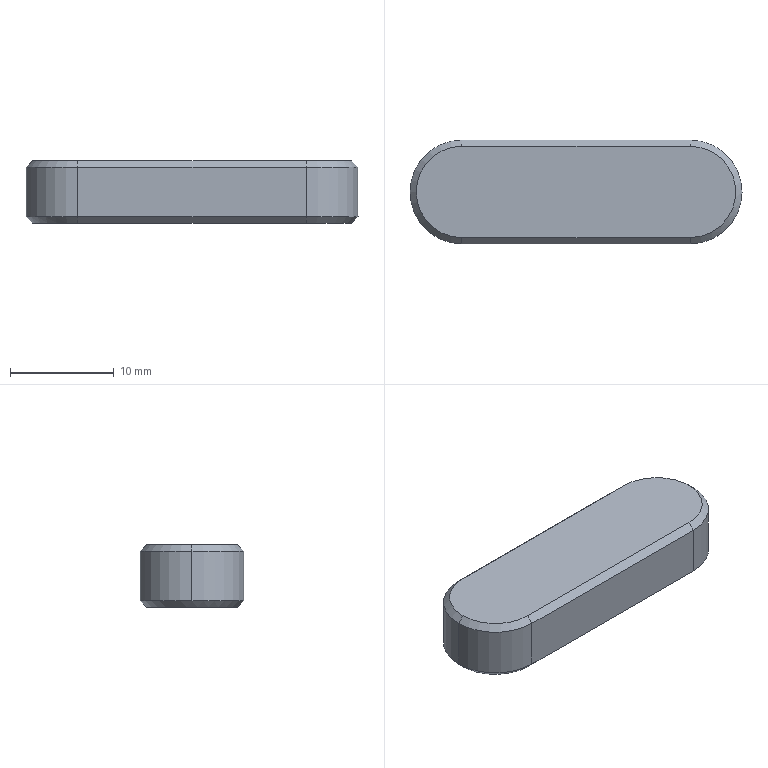Part | SolidWorks | features BaseBody 1 | 1 solid | 17 faces | box 32 x 10 x 6 mm | volume 1765 mm3 | plane 8 | cone 6 | cylinder 3 | commonest cylinder face diameters 10 x3
STEP:
#1=CARTESIAN_POINT('',(0.6,0.,2.5));
#2=VERTEX_POINT('',#1);
#3=CARTESIAN_POINT('',(5.,-4.4,2.5));
#4=VERTEX_POINT('',#3);
#5=CARTESIAN_POINT('',(5.,0.,2.5));
#6=DIRECTION('',(0.,0.,1.));
#7=DIRECTION('',(-1.,0.,0.));
#8=AXIS2_PLACEMENT_3D('',#5,#6,#7);
#9=CIRCLE('',#8,4.4);
#10=EDGE_CURVE('',#2,#4,#9,.T.);
#11=ORIENTED_EDGE('',*,*,#10,.F.);
#12=CARTESIAN_POINT('',(0.,0.,1.9));
#13=VERTEX_POINT('',#12);
#14=CARTESIAN_POINT('',(0.,0.,1.9));
#15=DIRECTION('',(-0.7071,0.,-0.7071));
#16=VECTOR('',#15,1000.);
#17=LINE('',#14,#16);
#18=EDGE_CURVE('',#2,#13,#17,.T.);
#19=ORIENTED_EDGE('',*,*,#18,.T.);
#20=CARTESIAN_POINT('',(5.,-5.,1.9));
#21=VERTEX_POINT('',#20);
#22=CARTESIAN_POINT('',(5.,0.,1.9));
#23=DIRECTION('',(0.,0.,1.));
#24=DIRECTION('',(0.,-1.,0.));
#25=AXIS2_PLACEMENT_3D('',#22,#23,#24);
#26=CIRCLE('',#25,5.);
#27=EDGE_CURVE('',#13,#21,#26,.T.);
#28=ORIENTED_EDGE('',*,*,#27,.T.);
#29=CARTESIAN_POINT('',(5.,-4.7,2.2));
#30=DIRECTION('',(0.,-0.7071,-0.7071));
#31=VECTOR('',#30,1000.);
#32=LINE('',#29,#31);
#33=EDGE_CURVE('',#4,#21,#32,.T.);
#34=ORIENTED_EDGE('',*,*,#33,.F.);
#35=EDGE_LOOP('',(#11,#19,#28,#34));
#36=FACE_OUTER_BOUND('',#35,.T.);
#37=CARTESIAN_POINT('',(5.,0.,1.9));
#38=DIRECTION('',(0.,0.,-1.));
#39=DIRECTION('',(-1.,0.,0.));
#40=AXIS2_PLACEMENT_3D('',#37,#38,#39);
#41=CONICAL_SURFACE('',#40,5.,0.7854);
#42=ADVANCED_FACE('',(#36),#41,.T.);
#43=ORIENTED_EDGE('',*,*,#27,.F.);
#44=CARTESIAN_POINT('',(0.,0.,-2.9));
#45=VERTEX_POINT('',#44);
#46=CARTESIAN_POINT('',(0.,0.,0.));
#47=DIRECTION('',(0.,0.,-1.));
#48=VECTOR('',#47,1000.);
#49=LINE('',#46,#48);
#50=EDGE_CURVE('',#13,#45,#49,.T.);
#51=ORIENTED_EDGE('',*,*,#50,.T.);
#52=CARTESIAN_POINT('',(5.,-5.,-2.9));
#53=VERTEX_POINT('',#52);
#54=CARTESIAN_POINT('',(5.,0.,-2.9));
#55=DIRECTION('',(0.,0.,1.));
#56=DIRECTION('',(-1.,0.,0.));
#57=AXIS2_PLACEMENT_3D('',#54,#55,#56);
#58=CIRCLE('',#57,5.);
#59=EDGE_CURVE('',#45,#53,#58,.T.);
#60=ORIENTED_EDGE('',*,*,#59,.T.);
#61=CARTESIAN_POINT('',(5.,-5.,0.));
#62=DIRECTION('',(0.,0.,-1.));
#63=VECTOR('',#62,1000.);
#64=LINE('',#61,#63);
#65=EDGE_CURVE('',#21,#53,#64,.T.);
#66=ORIENTED_EDGE('',*,*,#65,.F.);
#67=EDGE_LOOP('',(#43,#51,#60,#66));
#68=FACE_OUTER_BOUND('',#67,.T.);
#69=CARTESIAN_POINT('',(5.,0.,0.));
#70=DIRECTION('',(0.,0.,-1.));
#71=DIRECTION('',(-1.,0.,0.));
#72=AXIS2_PLACEMENT_3D('',#69,#70,#71);
#73=CYLINDRICAL_SURFACE('',#72,5.);
#74=ADVANCED_FACE('',(#68),#73,.T.);
#75=CARTESIAN_POINT('',(27.,-4.4,-3.5));
#76=VERTEX_POINT('',#75);
#77=CARTESIAN_POINT('',(31.4,0.,-3.5));
#78=VERTEX_POINT('',#77);
#79=CARTESIAN_POINT('',(27.,0.,-3.5));
#80=DIRECTION('',(0.,0.,1.));
#81=DIRECTION('',(1.,0.,0.));
#82=AXIS2_PLACEMENT_3D('',#79,#80,#81);
#83=CIRCLE('',#82,4.4);
#84=EDGE_CURVE('',#76,#78,#83,.T.);
#85=ORIENTED_EDGE('',*,*,#84,.T.);
#86=CARTESIAN_POINT('',(32.,0.,-2.9));
#87=VERTEX_POINT('',#86);
#88=CARTESIAN_POINT('',(32.,0.,-2.9));
#89=DIRECTION('',(0.7071,0.,0.7071));
#90=VECTOR('',#89,1000.);
#91=LINE('',#88,#90);
#92=EDGE_CURVE('',#78,#87,#91,.T.);
#93=ORIENTED_EDGE('',*,*,#92,.T.);
#94=CARTESIAN_POINT('',(27.,-5.,-2.9));
#95=VERTEX_POINT('',#94);
#96=CARTESIAN_POINT('',(27.,0.,-2.9));
#97=DIRECTION('',(0.,0.,1.));
#98=DIRECTION('',(-1.,0.,0.));
#99=AXIS2_PLACEMENT_3D('',#96,#97,#98);
#100=CIRCLE('',#99,5.);
#101=EDGE_CURVE('',#95,#87,#100,.T.);
#102=ORIENTED_EDGE('',*,*,#101,.F.);
#103=CARTESIAN_POINT('',(27.,-499000.,498992.1));
#104=DIRECTION('',(0.,0.7071,-0.7071));
#105=VECTOR('',#104,1000.);
#106=LINE('',#103,#105);
#107=EDGE_CURVE('',#95,#76,#106,.T.);
#108=ORIENTED_EDGE('',*,*,#107,.T.);
#109=EDGE_LOOP('',(#85,#93,#102,#108));
#110=FACE_OUTER_BOUND('',#109,.T.);
#111=CARTESIAN_POINT('',(27.,0.,-2.9));
#112=DIRECTION('',(0.,0.,1.));
#113=DIRECTION('',(1.,0.,0.));
#114=AXIS2_PLACEMENT_3D('',#111,#112,#113);
#115=CONICAL_SURFACE('',#114,5.,0.7854);
#116=ADVANCED_FACE('',(#110),#115,.T.);
#117=CARTESIAN_POINT('',(27.,-4.4,2.5));
#118=VERTEX_POINT('',#117);
#119=CARTESIAN_POINT('',(27.,4.4,2.5));
#120=VERTEX_POINT('',#119);
#121=CARTESIAN_POINT('',(27.,0.,2.5));
#122=DIRECTION('',(0.,0.,1.));
#123=DIRECTION('',(-1.,0.,0.));
#124=AXIS2_PLACEMENT_3D('',#121,#122,#123);
#125=CIRCLE('',#124,4.4);
#126=EDGE_CURVE('',#118,#120,#125,.T.);
#127=ORIENTED_EDGE('',*,*,#126,.T.);
#128=CARTESIAN_POINT('',(5.,4.4,2.5));
#129=VERTEX_POINT('',#128);
#130=CARTESIAN_POINT('',(16.,4.4,2.5));
#131=DIRECTION('',(-1.,0.,0.));
#132=VECTOR('',#131,1000.);
#133=LINE('',#130,#132);
#134=EDGE_CURVE('',#120,#129,#133,.T.);
#135=ORIENTED_EDGE('',*,*,#134,.T.);
#136=CARTESIAN_POINT('',(5.,0.,2.5));
#137=DIRECTION('',(0.,0.,1.));
#138=DIRECTION('',(-1.,0.,0.));
#139=AXIS2_PLACEMENT_3D('',#136,#137,#138);
#140=CIRCLE('',#139,4.4);
#141=EDGE_CURVE('',#129,#2,#140,.T.);
#142=ORIENTED_EDGE('',*,*,#141,.T.);
#143=ORIENTED_EDGE('',*,*,#10,.T.);
#144=CARTESIAN_POINT('',(16.,-4.4,2.5));
#145=DIRECTION('',(1.,0.,0.));
#146=VECTOR('',#145,1000.);
#147=LINE('',#144,#146);
#148=EDGE_CURVE('',#4,#118,#147,.T.);
#149=ORIENTED_EDGE('',*,*,#148,.T.);
#150=EDGE_LOOP('',(#127,#135,#142,#143,#149));
#151=FACE_OUTER_BOUND('',#150,.T.);
#152=CARTESIAN_POINT('',(16.,0.,2.5));
#153=DIRECTION('',(0.,0.,1.));
#154=DIRECTION('',(1.,0.,0.));
#155=AXIS2_PLACEMENT_3D('',#152,#153,#154);
#156=PLANE('',#155);
#157=ADVANCED_FACE('',(#151),#156,.T.);
#158=CARTESIAN_POINT('',(5.,5.,1.9));
#159=VERTEX_POINT('',#158);
#160=CARTESIAN_POINT('',(5.,4.7,2.2));
#161=DIRECTION('',(0.,-0.7071,0.7071));
#162=VECTOR('',#161,1000.);
#163=LINE('',#160,#162);
#164=EDGE_CURVE('',#159,#129,#163,.T.);
#165=ORIENTED_EDGE('',*,*,#164,.T.);
#166=ORIENTED_EDGE('',*,*,#134,.F.);
#167=CARTESIAN_POINT('',(27.,5.,1.9));
#168=VERTEX_POINT('',#167);
#169=CARTESIAN_POINT('',(27.,4.7,2.2));
#170=DIRECTION('',(0.,0.7071,-0.7071));
#171=VECTOR('',#170,1000.);
#172=LINE('',#169,#171);
#173=EDGE_CURVE('',#120,#168,#172,.T.);
#174=ORIENTED_EDGE('',*,*,#173,.T.);
#175=CARTESIAN_POINT('',(21.5,5.,1.9));
#176=DIRECTION('',(-1.,0.,0.));
#177=VECTOR('',#176,1000.);
#178=LINE('',#175,#177);
#179=EDGE_CURVE('',#168,#159,#178,.T.);
#180=ORIENTED_EDGE('',*,*,#179,.T.);
#181=EDGE_LOOP('',(#165,#166,#174,#180));
#182=FACE_OUTER_BOUND('',#181,.T.);
#183=CARTESIAN_POINT('',(21.5,4.7,2.2));
#184=DIRECTION('',(0.,0.7071,0.7071));
#185=DIRECTION('',(0.,-0.7071,0.7071));
#186=AXIS2_PLACEMENT_3D('',#183,#184,#185);
#187=PLANE('',#186);
#188=ADVANCED_FACE('',(#182),#187,.T.);
#189=ORIENTED_EDGE('',*,*,#173,.F.);
#190=ORIENTED_EDGE('',*,*,#126,.F.);
#191=CARTESIAN_POINT('',(27.,-5.,1.9));
#192=VERTEX_POINT('',#191);
#193=CARTESIAN_POINT('',(27.,-499000.,-498993.1));
#194=DIRECTION('',(0.,-0.7071,-0.7071));
#195=VECTOR('',#194,1000.);
#196=LINE('',#193,#195);
#197=EDGE_CURVE('',#118,#192,#196,.T.);
#198=ORIENTED_EDGE('',*,*,#197,.T.);
#199=CARTESIAN_POINT('',(27.,0.,1.9));
#200=DIRECTION('',(0.,0.,1.));
#201=DIRECTION('',(0.,1.,0.));
#202=AXIS2_PLACEMENT_3D('',#199,#200,#201);
#203=CIRCLE('',#202,5.);
#204=EDGE_CURVE('',#192,#168,#203,.T.);
#205=ORIENTED_EDGE('',*,*,#204,.T.);
#206=EDGE_LOOP('',(#189,#190,#198,#205));
#207=FACE_OUTER_BOUND('',#206,.T.);
#208=CARTESIAN_POINT('',(27.,0.,1.9));
#209=DIRECTION('',(0.,0.,-1.));
#210=DIRECTION('',(-1.,0.,0.));
#211=AXIS2_PLACEMENT_3D('',#208,#209,#210);
#212=CONICAL_SURFACE('',#211,5.,0.7854);
#213=ADVANCED_FACE('',(#207),#212,.T.);
#214=ORIENTED_EDGE('',*,*,#33,.T.);
#215=CARTESIAN_POINT('',(10.5,-5.,1.9));
#216=DIRECTION('',(1.,0.,0.));
#217=VECTOR('',#216,1000.);
#218=LINE('',#215,#217);
#219=EDGE_CURVE('',#21,#192,#218,.T.);
#220=ORIENTED_EDGE('',*,*,#219,.T.);
#221=ORIENTED_EDGE('',*,*,#197,.F.);
#222=ORIENTED_EDGE('',*,*,#148,.F.);
#223=EDGE_LOOP('',(#214,#220,#221,#222));
#224=FACE_OUTER_BOUND('',#223,.T.);
#225=CARTESIAN_POINT('',(10.5,-4.7,2.2));
#226=DIRECTION('',(0.,-0.7071,0.7071));
#227=DIRECTION('',(0.,-0.7071,-0.7071));
#228=AXIS2_PLACEMENT_3D('',#225,#226,#227);
#229=PLANE('',#228);
#230=ADVANCED_FACE('',(#224),#229,.T.);
#231=ORIENTED_EDGE('',*,*,#18,.F.);
#232=ORIENTED_EDGE('',*,*,#141,.F.);
#233=ORIENTED_EDGE('',*,*,#164,.F.);
#234=CARTESIAN_POINT('',(5.,0.,1.9));
#235=DIRECTION('',(0.,0.,1.));
#236=DIRECTION('',(0.,-1.,0.));
#237=AXIS2_PLACEMENT_3D('',#234,#235,#236);
#238=CIRCLE('',#237,5.);
#239=EDGE_CURVE('',#159,#13,#238,.T.);
#240=ORIENTED_EDGE('',*,*,#239,.T.);
#241=EDGE_LOOP('',(#231,#232,#233,#240));
#242=FACE_OUTER_BOUND('',#241,.T.);
#243=CARTESIAN_POINT('',(5.,0.,1.9));
#244=DIRECTION('',(0.,0.,-1.));
#245=DIRECTION('',(-1.,0.,0.));
#246=AXIS2_PLACEMENT_3D('',#243,#244,#245);
#247=CONICAL_SURFACE('',#246,5.,0.7854);
#248=ADVANCED_FACE('',(#242),#247,.T.);
#249=ORIENTED_EDGE('',*,*,#179,.F.);
#250=CARTESIAN_POINT('',(27.,5.,-2.9));
#251=VERTEX_POINT('',#250);
#252=CARTESIAN_POINT('',(27.,5.,0.));
#253=DIRECTION('',(0.,0.,-1.));
#254=VECTOR('',#253,1000.);
#255=LINE('',#252,#254);
#256=EDGE_CURVE('',#168,#251,#255,.T.);
#257=ORIENTED_EDGE('',*,*,#256,.T.);
#258=CARTESIAN_POINT('',(5.,5.,-2.9));
#259=VERTEX_POINT('',#258);
#260=CARTESIAN_POINT('',(27.,5.,-2.9));
#261=DIRECTION('',(-1.,0.,0.));
#262=VECTOR('',#261,1000.);
#263=LINE('',#260,#262);
#264=EDGE_CURVE('',#251,#259,#263,.T.);
#265=ORIENTED_EDGE('',*,*,#264,.T.);
#266=CARTESIAN_POINT('',(5.,5.,0.));
#267=DIRECTION('',(0.,0.,1.));
#268=VECTOR('',#267,1000.);
#269=LINE('',#266,#268);
#270=EDGE_CURVE('',#259,#159,#269,.T.);
#271=ORIENTED_EDGE('',*,*,#270,.T.);
#272=EDGE_LOOP('',(#249,#257,#265,#271));
#273=FACE_OUTER_BOUND('',#272,.T.);
#274=CARTESIAN_POINT('',(27.,5.,0.));
#275=DIRECTION('',(0.,1.,0.));
#276=DIRECTION('',(0.,0.,1.));
#277=AXIS2_PLACEMENT_3D('',#274,#275,#276);
#278=PLANE('',#277);
#279=ADVANCED_FACE('',(#273),#278,.T.);
#280=ORIENTED_EDGE('',*,*,#204,.F.);
#281=CARTESIAN_POINT('',(27.,-5.,0.));
#282=DIRECTION('',(0.,0.,-1.));
#283=VECTOR('',#282,1000.);
#284=LINE('',#281,#283);
#285=EDGE_CURVE('',#192,#95,#284,.T.);
#286=ORIENTED_EDGE('',*,*,#285,.T.);
#287=ORIENTED_EDGE('',*,*,#101,.T.);
#288=CARTESIAN_POINT('',(27.,0.,-2.9));
#289=DIRECTION('',(0.,0.,1.));
#290=DIRECTION('',(-1.,0.,0.));
#291=AXIS2_PLACEMENT_3D('',#288,#289,#290);
#292=CIRCLE('',#291,5.);
#293=EDGE_CURVE('',#87,#251,#292,.T.);
#294=ORIENTED_EDGE('',*,*,#293,.T.);
#295=ORIENTED_EDGE('',*,*,#256,.F.);
#296=EDGE_LOOP('',(#280,#286,#287,#294,#295));
#297=FACE_OUTER_BOUND('',#296,.T.);
#298=CARTESIAN_POINT('',(27.,0.,0.));
#299=DIRECTION('',(0.,0.,-1.));
#300=DIRECTION('',(-1.,0.,0.));
#301=AXIS2_PLACEMENT_3D('',#298,#299,#300);
#302=CYLINDRICAL_SURFACE('',#301,5.);
#303=ADVANCED_FACE('',(#297),#302,.T.);
#304=ORIENTED_EDGE('',*,*,#219,.F.);
#305=ORIENTED_EDGE('',*,*,#65,.T.);
#306=CARTESIAN_POINT('',(5.,-5.,-2.9));
#307=DIRECTION('',(1.,0.,0.));
#308=VECTOR('',#307,1000.);
#309=LINE('',#306,#308);
#310=EDGE_CURVE('',#53,#95,#309,.T.);
#311=ORIENTED_EDGE('',*,*,#310,.T.);
#312=ORIENTED_EDGE('',*,*,#285,.F.);
#313=EDGE_LOOP('',(#304,#305,#311,#312));
#314=FACE_OUTER_BOUND('',#313,.T.);
#315=CARTESIAN_POINT('',(5.,-5.,0.));
#316=DIRECTION('',(0.,-1.,0.));
#317=DIRECTION('',(1.,0.,0.));
#318=AXIS2_PLACEMENT_3D('',#315,#316,#317);
#319=PLANE('',#318);
#320=ADVANCED_FACE('',(#314),#319,.T.);
#321=ORIENTED_EDGE('',*,*,#50,.F.);
#322=ORIENTED_EDGE('',*,*,#239,.F.);
#323=ORIENTED_EDGE('',*,*,#270,.F.);
#324=CARTESIAN_POINT('',(5.,0.,-2.9));
#325=DIRECTION('',(0.,0.,1.));
#326=DIRECTION('',(-1.,0.,0.));
#327=AXIS2_PLACEMENT_3D('',#324,#325,#326);
#328=CIRCLE('',#327,5.);
#329=EDGE_CURVE('',#259,#45,#328,.T.);
#330=ORIENTED_EDGE('',*,*,#329,.T.);
#331=EDGE_LOOP('',(#321,#322,#323,#330));
#332=FACE_OUTER_BOUND('',#331,.T.);
#333=CARTESIAN_POINT('',(5.,0.,0.));
#334=DIRECTION('',(0.,0.,-1.));
#335=DIRECTION('',(-1.,0.,0.));
#336=AXIS2_PLACEMENT_3D('',#333,#334,#335);
#337=CYLINDRICAL_SURFACE('',#336,5.);
#338=ADVANCED_FACE('',(#332),#337,.T.);
#339=CARTESIAN_POINT('',(5.,4.4,-3.5));
#340=VERTEX_POINT('',#339);
#341=CARTESIAN_POINT('',(5.,4.7,-3.2));
#342=DIRECTION('',(0.,0.7071,0.7071));
#343=VECTOR('',#342,1000.);
#344=LINE('',#341,#343);
#345=EDGE_CURVE('',#340,#259,#344,.T.);
#346=ORIENTED_EDGE('',*,*,#345,.T.);
#347=ORIENTED_EDGE('',*,*,#264,.F.);
#348=CARTESIAN_POINT('',(27.,4.4,-3.5));
#349=VERTEX_POINT('',#348);
#350=CARTESIAN_POINT('',(27.,4.7,-3.2));
#351=DIRECTION('',(0.,-0.7071,-0.7071));
#352=VECTOR('',#351,1000.);
#353=LINE('',#350,#352);
#354=EDGE_CURVE('',#251,#349,#353,.T.);
#355=ORIENTED_EDGE('',*,*,#354,.T.);
#356=CARTESIAN_POINT('',(21.5,4.4,-3.5));
#357=DIRECTION('',(-1.,0.,0.));
#358=VECTOR('',#357,1000.);
#359=LINE('',#356,#358);
#360=EDGE_CURVE('',#349,#340,#359,.T.);
#361=ORIENTED_EDGE('',*,*,#360,.T.);
#362=EDGE_LOOP('',(#346,#347,#355,#361));
#363=FACE_OUTER_BOUND('',#362,.T.);
#364=CARTESIAN_POINT('',(21.5,4.7,-3.2));
#365=DIRECTION('',(0.,0.7071,-0.7071));
#366=DIRECTION('',(0.,0.7071,0.7071));
#367=AXIS2_PLACEMENT_3D('',#364,#365,#366);
#368=PLANE('',#367);
#369=ADVANCED_FACE('',(#363),#368,.T.);
#370=ORIENTED_EDGE('',*,*,#92,.F.);
#371=CARTESIAN_POINT('',(27.,0.,-3.5));
#372=DIRECTION('',(0.,0.,1.));
#373=DIRECTION('',(1.,0.,0.));
#374=AXIS2_PLACEMENT_3D('',#371,#372,#373);
#375=CIRCLE('',#374,4.4);
#376=EDGE_CURVE('',#78,#349,#375,.T.);
#377=ORIENTED_EDGE('',*,*,#376,.T.);
#378=ORIENTED_EDGE('',*,*,#354,.F.);
#379=ORIENTED_EDGE('',*,*,#293,.F.);
#380=EDGE_LOOP('',(#370,#377,#378,#379));
#381=FACE_OUTER_BOUND('',#380,.T.);
#382=CARTESIAN_POINT('',(27.,0.,-2.9));
#383=DIRECTION('',(0.,0.,1.));
#384=DIRECTION('',(1.,0.,0.));
#385=AXIS2_PLACEMENT_3D('',#382,#383,#384);
#386=CONICAL_SURFACE('',#385,5.,0.7854);
#387=ADVANCED_FACE('',(#381),#386,.T.);
#388=CARTESIAN_POINT('',(5.,-4.4,-3.5));
#389=VERTEX_POINT('',#388);
#390=CARTESIAN_POINT('',(5.,-4.7,-3.2));
#391=DIRECTION('',(0.,0.7071,-0.7071));
#392=VECTOR('',#391,1000.);
#393=LINE('',#390,#392);
#394=EDGE_CURVE('',#53,#389,#393,.T.);
#395=ORIENTED_EDGE('',*,*,#394,.T.);
#396=CARTESIAN_POINT('',(10.5,-4.4,-3.5));
#397=DIRECTION('',(1.,0.,0.));
#398=VECTOR('',#397,1000.);
#399=LINE('',#396,#398);
#400=EDGE_CURVE('',#389,#76,#399,.T.);
#401=ORIENTED_EDGE('',*,*,#400,.T.);
#402=ORIENTED_EDGE('',*,*,#107,.F.);
#403=ORIENTED_EDGE('',*,*,#310,.F.);
#404=EDGE_LOOP('',(#395,#401,#402,#403));
#405=FACE_OUTER_BOUND('',#404,.T.);
#406=CARTESIAN_POINT('',(10.5,-4.7,-3.2));
#407=DIRECTION('',(0.,-0.7071,-0.7071));
#408=DIRECTION('',(0.,0.7071,-0.7071));
#409=AXIS2_PLACEMENT_3D('',#406,#407,#408);
#410=PLANE('',#409);
#411=ADVANCED_FACE('',(#405),#410,.T.);
#412=ORIENTED_EDGE('',*,*,#394,.F.);
#413=ORIENTED_EDGE('',*,*,#59,.F.);
#414=ORIENTED_EDGE('',*,*,#329,.F.);
#415=ORIENTED_EDGE('',*,*,#345,.F.);
#416=CARTESIAN_POINT('',(5.,0.,-3.5));
#417=DIRECTION('',(0.,0.,1.));
#418=DIRECTION('',(1.,0.,0.));
#419=AXIS2_PLACEMENT_3D('',#416,#417,#418);
#420=CIRCLE('',#419,4.4);
#421=EDGE_CURVE('',#340,#389,#420,.T.);
#422=ORIENTED_EDGE('',*,*,#421,.T.);
#423=EDGE_LOOP('',(#412,#413,#414,#415,#422));
#424=FACE_OUTER_BOUND('',#423,.T.);
#425=CARTESIAN_POINT('',(5.,0.,-2.9));
#426=DIRECTION('',(0.,0.,1.));
#427=DIRECTION('',(1.,0.,0.));
#428=AXIS2_PLACEMENT_3D('',#425,#426,#427);
#429=CONICAL_SURFACE('',#428,5.,0.7854);
#430=ADVANCED_FACE('',(#424),#429,.T.);
#431=ORIENTED_EDGE('',*,*,#421,.F.);
#432=ORIENTED_EDGE('',*,*,#360,.F.);
#433=ORIENTED_EDGE('',*,*,#376,.F.);
#434=ORIENTED_EDGE('',*,*,#84,.F.);
#435=ORIENTED_EDGE('',*,*,#400,.F.);
#436=EDGE_LOOP('',(#431,#432,#433,#434,#435));
#437=FACE_OUTER_BOUND('',#436,.T.);
#438=CARTESIAN_POINT('',(16.,0.,-3.5));
#439=DIRECTION('',(0.,0.,1.));
#440=DIRECTION('',(1.,0.,0.));
#441=AXIS2_PLACEMENT_3D('',#438,#439,#440);
#442=PLANE('',#441);
#443=ADVANCED_FACE('',(#437),#442,.F.);
#444=CLOSED_SHELL('',(#42,#74,#116,#157,#188,#213,#230,#248,#279,#303,#320,#338,#369,#387,#411,#430,#443));
#445=MANIFOLD_SOLID_BREP('',#444);
#446=CARTESIAN_POINT('',(0.,0.,0.));
#447=DIRECTION('',(0.,0.,1.));
#448=DIRECTION('',(1.,0.,0.));
#449=AXIS2_PLACEMENT_3D('',#446,#447,#448);
#450=(LENGTH_UNIT()NAMED_UNIT(*)SI_UNIT(.MILLI.,.METRE.));
#451=UNCERTAINTY_MEASURE_WITH_UNIT(LENGTH_MEASURE(0.00001),#450,'','');
#452=(NAMED_UNIT(*)PLANE_ANGLE_UNIT()SI_UNIT($,.RADIAN.));
#453=(NAMED_UNIT(*)SI_UNIT($,.STERADIAN.)SOLID_ANGLE_UNIT());
#454=(GEOMETRIC_REPRESENTATION_CONTEXT(3)GLOBAL_UNCERTAINTY_ASSIGNED_CONTEXT((#451))GLOBAL_UNIT_ASSIGNED_CONTEXT((#450,#452,#453))REPRESENTATION_CONTEXT('',''));
#455=ADVANCED_BREP_SHAPE_REPRESENTATION('',(#445,#449),#454);